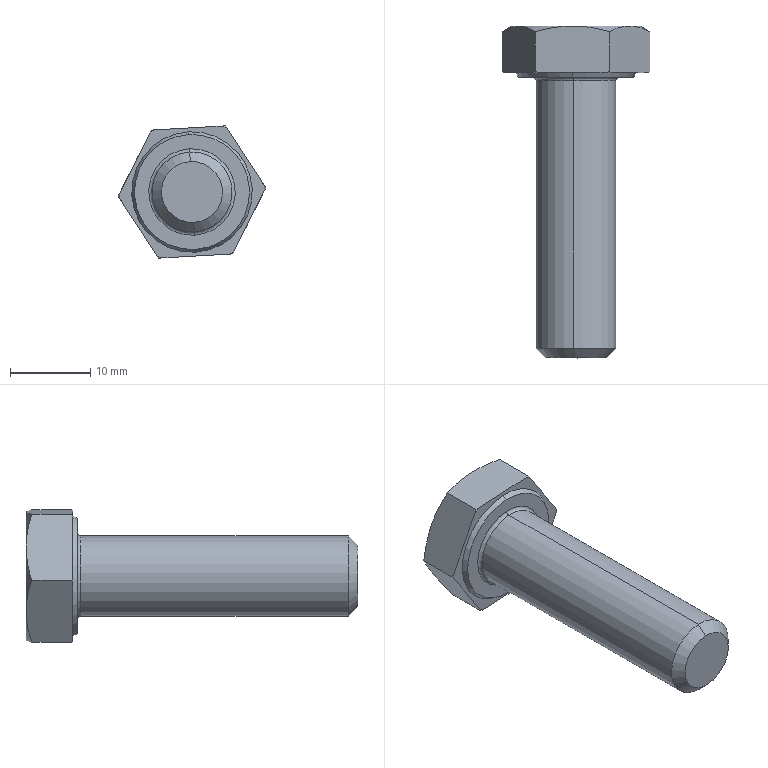Part | STEP file | BFACE2-39 | 1 solid | 30 faces | box 18.445 x 41.4 x 16.5 mm | volume 4112 mm3 | cone 16 | plane 10 | cylinder 2 | torus 2 | commonest cylinder face diameters 10 x2
STEP:
#1=CARTESIAN_POINT('',(-602.523,-427.673,3364.161));
#2=VERTEX_POINT('',#1);
#3=CARTESIAN_POINT('',(-601.954,-427.673,3354.177));
#4=VERTEX_POINT('',#3);
#5=CARTESIAN_POINT('',(-602.238,-427.673,3359.169));
#6=DIRECTION('',(0.,1.,0.));
#7=DIRECTION('',(-0.05688,0.,0.9984));
#8=AXIS2_PLACEMENT_3D('',#5,#6,#7);
#9=CIRCLE('',#8,5.);
#10=EDGE_CURVE('',#2,#4,#9,.T.);
#11=ORIENTED_EDGE('',*,*,#10,.F.);
#12=CARTESIAN_POINT('',(-602.523,-461.073,3364.161));
#13=VERTEX_POINT('',#12);
#14=CARTESIAN_POINT('',(-602.523,-420.873,3364.161));
#15=DIRECTION('',(0.,1.,0.));
#16=VECTOR('',#15,1000.);
#17=LINE('',#14,#16);
#18=EDGE_CURVE('',#13,#2,#17,.T.);
#19=ORIENTED_EDGE('',*,*,#18,.F.);
#20=CARTESIAN_POINT('',(-601.954,-461.073,3354.177));
#21=VERTEX_POINT('',#20);
#22=CARTESIAN_POINT('',(-602.238,-461.073,3359.169));
#23=DIRECTION('',(0.,1.,0.));
#24=DIRECTION('',(0.05688,0.,-0.9984));
#25=AXIS2_PLACEMENT_3D('',#22,#23,#24);
#26=CIRCLE('',#25,5.);
#27=EDGE_CURVE('',#13,#21,#26,.T.);
#28=ORIENTED_EDGE('',*,*,#27,.T.);
#29=CARTESIAN_POINT('',(-601.954,-420.873,3354.177));
#30=DIRECTION('',(0.,1.,0.));
#31=VECTOR('',#30,1000.);
#32=LINE('',#29,#31);
#33=EDGE_CURVE('',#21,#4,#32,.T.);
#34=ORIENTED_EDGE('',*,*,#33,.T.);
#35=EDGE_LOOP('',(#11,#19,#28,#34));
#36=FACE_OUTER_BOUND('',#35,.T.);
#37=CARTESIAN_POINT('',(-602.238,-420.873,3359.169));
#38=DIRECTION('',(0.,-1.,0.));
#39=DIRECTION('',(-0.05688,0.,0.9984));
#40=AXIS2_PLACEMENT_3D('',#37,#38,#39);
#41=CYLINDRICAL_SURFACE('',#40,5.);
#42=ADVANCED_FACE('',(#36),#41,.T.);
#43=CARTESIAN_POINT('',(-602.022,-462.273,3355.375));
#44=VERTEX_POINT('',#43);
#45=CARTESIAN_POINT('',(-602.454,-462.273,3362.963));
#46=VERTEX_POINT('',#45);
#47=CARTESIAN_POINT('',(-602.238,-462.273,3359.169));
#48=DIRECTION('',(0.,-1.,0.));
#49=DIRECTION('',(0.05688,0.,-0.9984));
#50=AXIS2_PLACEMENT_3D('',#47,#48,#49);
#51=CIRCLE('',#50,3.8);
#52=EDGE_CURVE('',#44,#46,#51,.T.);
#53=ORIENTED_EDGE('',*,*,#52,.F.);
#54=CARTESIAN_POINT('',(-602.022,-462.273,3355.375));
#55=DIRECTION('',(0.04022,0.7071,-0.706));
#56=VECTOR('',#55,1000.);
#57=LINE('',#54,#56);
#58=EDGE_CURVE('',#44,#21,#57,.T.);
#59=ORIENTED_EDGE('',*,*,#58,.T.);
#60=ORIENTED_EDGE('',*,*,#27,.F.);
#61=CARTESIAN_POINT('',(-602.454,-462.273,3362.963));
#62=DIRECTION('',(-0.04022,0.7071,0.706));
#63=VECTOR('',#62,1000.);
#64=LINE('',#61,#63);
#65=EDGE_CURVE('',#46,#13,#64,.T.);
#66=ORIENTED_EDGE('',*,*,#65,.F.);
#67=EDGE_LOOP('',(#53,#59,#60,#66));
#68=FACE_OUTER_BOUND('',#67,.T.);
#69=CARTESIAN_POINT('',(-602.238,-462.273,3359.169));
#70=DIRECTION('',(0.,1.,0.));
#71=DIRECTION('',(0.05688,0.,-0.9984));
#72=AXIS2_PLACEMENT_3D('',#69,#70,#71);
#73=CONICAL_SURFACE('',#72,3.8,0.7854);
#74=ADVANCED_FACE('',(#68),#73,.T.);
#75=CARTESIAN_POINT('',(-601.931,-427.273,3353.778));
#76=VERTEX_POINT('',#75);
#77=CARTESIAN_POINT('',(-602.545,-427.273,3364.56));
#78=VERTEX_POINT('',#77);
#79=CARTESIAN_POINT('',(-602.238,-427.273,3359.169));
#80=DIRECTION('',(0.,1.,0.));
#81=DIRECTION('',(-0.05688,0.,0.9984));
#82=AXIS2_PLACEMENT_3D('',#79,#80,#81);
#83=CIRCLE('',#82,5.4);
#84=EDGE_CURVE('',#76,#78,#83,.T.);
#85=ORIENTED_EDGE('',*,*,#84,.F.);
#86=CARTESIAN_POINT('',(-601.931,-427.673,3353.778));
#87=DIRECTION('',(0.9984,0.,0.05688));
#88=DIRECTION('',(-0.05688,0.,0.9984));
#89=AXIS2_PLACEMENT_3D('',#86,#87,#88);
#90=CIRCLE('',#89,0.4);
#91=EDGE_CURVE('',#76,#4,#90,.T.);
#92=ORIENTED_EDGE('',*,*,#91,.T.);
#93=CARTESIAN_POINT('',(-602.238,-427.673,3359.169));
#94=DIRECTION('',(0.,1.,0.));
#95=DIRECTION('',(-0.05688,0.,0.9984));
#96=AXIS2_PLACEMENT_3D('',#93,#94,#95);
#97=CIRCLE('',#96,5.);
#98=EDGE_CURVE('',#4,#2,#97,.T.);
#99=ORIENTED_EDGE('',*,*,#98,.T.);
#100=CARTESIAN_POINT('',(-602.545,-427.673,3364.56));
#101=DIRECTION('',(-0.9984,0.,-0.05688));
#102=DIRECTION('',(0.05688,0.,-0.9984));
#103=AXIS2_PLACEMENT_3D('',#100,#101,#102);
#104=CIRCLE('',#103,0.4);
#105=EDGE_CURVE('',#78,#2,#104,.T.);
#106=ORIENTED_EDGE('',*,*,#105,.F.);
#107=EDGE_LOOP('',(#85,#92,#99,#106));
#108=FACE_OUTER_BOUND('',#107,.T.);
#109=CARTESIAN_POINT('',(-602.238,-427.673,3359.169));
#110=DIRECTION('',(0.,1.,0.));
#111=DIRECTION('',(0.05688,0.,-0.9984));
#112=AXIS2_PLACEMENT_3D('',#109,#110,#111);
#113=TOROIDAL_SURFACE('',#112,5.4,0.4);
#114=ADVANCED_FACE('',(#108),#113,.F.);
#115=CARTESIAN_POINT('',(-602.647,-427.273,3366.335));
#116=VERTEX_POINT('',#115);
#117=CARTESIAN_POINT('',(-601.83,-427.273,3352.003));
#118=VERTEX_POINT('',#117);
#119=CARTESIAN_POINT('',(-602.238,-427.273,3359.169));
#120=DIRECTION('',(0.,1.,0.));
#121=DIRECTION('',(-0.05688,0.,0.9984));
#122=AXIS2_PLACEMENT_3D('',#119,#120,#121);
#123=CIRCLE('',#122,7.177);
#124=EDGE_CURVE('',#116,#118,#123,.T.);
#125=ORIENTED_EDGE('',*,*,#124,.T.);
#126=CARTESIAN_POINT('',(-601.81,-426.673,3351.658));
#127=VERTEX_POINT('',#126);
#128=CARTESIAN_POINT('',(-601.81,-426.673,3351.658));
#129=DIRECTION('',(0.02844,0.866,-0.4992));
#130=VECTOR('',#129,1000.);
#131=LINE('',#128,#130);
#132=EDGE_CURVE('',#118,#127,#131,.T.);
#133=ORIENTED_EDGE('',*,*,#132,.T.);
#134=CARTESIAN_POINT('',(-602.666,-426.673,3366.681));
#135=VERTEX_POINT('',#134);
#136=CARTESIAN_POINT('',(-602.238,-426.673,3359.169));
#137=DIRECTION('',(0.,1.,0.));
#138=DIRECTION('',(-0.05688,0.,0.9984));
#139=AXIS2_PLACEMENT_3D('',#136,#137,#138);
#140=CIRCLE('',#139,7.524);
#141=EDGE_CURVE('',#135,#127,#140,.T.);
#142=ORIENTED_EDGE('',*,*,#141,.F.);
#143=CARTESIAN_POINT('',(-602.666,-426.673,3366.681));
#144=DIRECTION('',(-0.02844,0.866,0.4992));
#145=VECTOR('',#144,1000.);
#146=LINE('',#143,#145);
#147=EDGE_CURVE('',#116,#135,#146,.T.);
#148=ORIENTED_EDGE('',*,*,#147,.F.);
#149=EDGE_LOOP('',(#125,#133,#142,#148));
#150=FACE_OUTER_BOUND('',#149,.T.);
#151=CARTESIAN_POINT('',(-602.238,-426.673,3359.169));
#152=DIRECTION('',(0.,1.,0.));
#153=DIRECTION('',(0.05688,0.,-0.9984));
#154=AXIS2_PLACEMENT_3D('',#151,#152,#153);
#155=CONICAL_SURFACE('',#154,7.524,0.5236);
#156=ADVANCED_FACE('',(#150),#155,.T.);
#157=ORIENTED_EDGE('',*,*,#124,.F.);
#158=CARTESIAN_POINT('',(-602.238,-427.273,3359.169));
#159=DIRECTION('',(0.,1.,0.));
#160=DIRECTION('',(-0.05688,0.,0.9984));
#161=AXIS2_PLACEMENT_3D('',#158,#159,#160);
#162=CIRCLE('',#161,7.177);
#163=EDGE_CURVE('',#118,#116,#162,.T.);
#164=ORIENTED_EDGE('',*,*,#163,.F.);
#165=EDGE_LOOP('',(#157,#164));
#166=FACE_OUTER_BOUND('',#165,.T.);
#167=CARTESIAN_POINT('',(-602.238,-427.273,3359.169));
#168=DIRECTION('',(0.,1.,0.));
#169=DIRECTION('',(-0.05688,0.,0.9984));
#170=AXIS2_PLACEMENT_3D('',#167,#168,#169);
#171=CIRCLE('',#170,5.4);
#172=EDGE_CURVE('',#78,#76,#171,.T.);
#173=ORIENTED_EDGE('',*,*,#172,.T.);
#174=ORIENTED_EDGE('',*,*,#84,.T.);
#175=EDGE_LOOP('',(#173,#174));
#176=FACE_BOUND('',#175,.T.);
#177=CARTESIAN_POINT('',(-593.016,-427.273,3359.695));
#178=DIRECTION('',(0.,-1.,0.));
#179=DIRECTION('',(-0.05688,0.,0.9984));
#180=AXIS2_PLACEMENT_3D('',#177,#178,#179);
#181=PLANE('',#180);
#182=ADVANCED_FACE('',(#166,#176),#181,.T.);
#183=CARTESIAN_POINT('',(-596.987,-426.673,3351.812));
#184=VERTEX_POINT('',#183);
#185=CARTESIAN_POINT('',(-593.2,-426.673,3359.328));
#186=VERTEX_POINT('',#185);
#187=CARTESIAN_POINT('',(-597.172,-426.673,3351.445));
#188=DIRECTION('',(0.4499,0.,0.8931));
#189=VECTOR('',#188,1000.);
#190=LINE('',#187,#189);
#191=EDGE_CURVE('',#184,#186,#190,.T.);
#192=ORIENTED_EDGE('',*,*,#191,.F.);
#193=CARTESIAN_POINT('',(-597.172,-426.559,3351.445));
#194=VERTEX_POINT('',#193);
#195=CARTESIAN_POINT('',(-597.172,-426.559,3351.445));
#196=CARTESIAN_POINT('',(-597.11,-426.598,3351.567));
#197=CARTESIAN_POINT('',(-597.049,-426.636,3351.689));
#198=CARTESIAN_POINT('',(-596.987,-426.673,3351.812));
#199=B_SPLINE_CURVE_WITH_KNOTS('',3,(#195,#196,#197,#198),.UNSPECIFIED.,.F.,.F.,(4,4),(0.,1.),.UNSPECIFIED.);
#200=EDGE_CURVE('',#194,#184,#199,.T.);
#201=ORIENTED_EDGE('',*,*,#200,.F.);
#202=CARTESIAN_POINT('',(-597.172,-421.588,3351.445));
#203=VERTEX_POINT('',#202);
#204=CARTESIAN_POINT('',(-597.172,-427.273,3351.445));
#205=DIRECTION('',(0.,1.,0.));
#206=VECTOR('',#205,1000.);
#207=LINE('',#204,#206);
#208=EDGE_CURVE('',#194,#203,#207,.T.);
#209=ORIENTED_EDGE('',*,*,#208,.T.);
#210=CARTESIAN_POINT('',(-595.094,-420.873,3355.57));
#211=VERTEX_POINT('',#210);
#212=CARTESIAN_POINT('',(-595.094,-420.873,3355.57));
#213=CARTESIAN_POINT('',(-595.448,-420.873,3354.866));
#214=CARTESIAN_POINT('',(-595.798,-420.941,3354.171));
#215=CARTESIAN_POINT('',(-596.49,-421.19,3352.798));
#216=CARTESIAN_POINT('',(-596.832,-421.37,3352.119));
#217=CARTESIAN_POINT('',(-597.172,-421.588,3351.445));
#218=B_SPLINE_CURVE_WITH_KNOTS('',3,(#212,#213,#214,#215,#216,#217),.UNSPECIFIED.,.F.,.F.,(4,2,4),(0.,0.002337,0.004674),.UNSPECIFIED.);
#219=EDGE_CURVE('',#211,#203,#218,.T.);
#220=ORIENTED_EDGE('',*,*,#219,.F.);
#221=CARTESIAN_POINT('',(-593.016,-421.588,3359.695));
#222=VERTEX_POINT('',#221);
#223=CARTESIAN_POINT('',(-593.016,-421.588,3359.695));
#224=CARTESIAN_POINT('',(-593.355,-421.37,3359.021));
#225=CARTESIAN_POINT('',(-593.697,-421.19,3358.342));
#226=CARTESIAN_POINT('',(-594.389,-420.941,3356.968));
#227=CARTESIAN_POINT('',(-594.739,-420.873,3356.274));
#228=CARTESIAN_POINT('',(-595.094,-420.873,3355.57));
#229=B_SPLINE_CURVE_WITH_KNOTS('',3,(#223,#224,#225,#226,#227,#228),.UNSPECIFIED.,.F.,.F.,(4,2,4),(0.,0.002337,0.004674),.UNSPECIFIED.);
#230=EDGE_CURVE('',#222,#211,#229,.T.);
#231=ORIENTED_EDGE('',*,*,#230,.F.);
#232=CARTESIAN_POINT('',(-593.016,-426.559,3359.695));
#233=VERTEX_POINT('',#232);
#234=CARTESIAN_POINT('',(-593.016,-427.273,3359.695));
#235=DIRECTION('',(0.,1.,0.));
#236=VECTOR('',#235,1000.);
#237=LINE('',#234,#236);
#238=EDGE_CURVE('',#233,#222,#237,.T.);
#239=ORIENTED_EDGE('',*,*,#238,.F.);
#240=CARTESIAN_POINT('',(-593.2,-426.673,3359.328));
#241=CARTESIAN_POINT('',(-593.139,-426.636,3359.45));
#242=CARTESIAN_POINT('',(-593.077,-426.598,3359.572));
#243=CARTESIAN_POINT('',(-593.016,-426.559,3359.695));
#244=B_SPLINE_CURVE_WITH_KNOTS('',3,(#240,#241,#242,#243),.UNSPECIFIED.,.F.,.F.,(4,4),(0.,1.),.UNSPECIFIED.);
#245=EDGE_CURVE('',#186,#233,#244,.T.);
#246=ORIENTED_EDGE('',*,*,#245,.F.);
#247=EDGE_LOOP('',(#192,#201,#209,#220,#231,#239,#246));
#248=FACE_OUTER_BOUND('',#247,.T.);
#249=CARTESIAN_POINT('',(-597.172,-427.273,3351.445));
#250=DIRECTION('',(-0.8931,0.,0.4499));
#251=DIRECTION('',(0.4499,0.,0.8931));
#252=AXIS2_PLACEMENT_3D('',#249,#250,#251);
#253=PLANE('',#252);
#254=ADVANCED_FACE('',(#248),#253,.F.);
#255=CARTESIAN_POINT('',(-593.241,-426.673,3360.038));
#256=VERTEX_POINT('',#255);
#257=CARTESIAN_POINT('',(-597.857,-426.673,3367.075));
#258=VERTEX_POINT('',#257);
#259=CARTESIAN_POINT('',(-593.016,-426.673,3359.695));
#260=DIRECTION('',(-0.5485,0.,0.8362));
#261=VECTOR('',#260,1000.);
#262=LINE('',#259,#261);
#263=EDGE_CURVE('',#256,#258,#262,.T.);
#264=ORIENTED_EDGE('',*,*,#263,.F.);
#265=CARTESIAN_POINT('',(-593.016,-426.559,3359.695));
#266=CARTESIAN_POINT('',(-593.091,-426.598,3359.809));
#267=CARTESIAN_POINT('',(-593.166,-426.636,3359.923));
#268=CARTESIAN_POINT('',(-593.241,-426.673,3360.038));
#269=B_SPLINE_CURVE_WITH_KNOTS('',3,(#265,#266,#267,#268),.UNSPECIFIED.,.F.,.F.,(4,4),(0.,1.),.UNSPECIFIED.);
#270=EDGE_CURVE('',#233,#256,#269,.T.);
#271=ORIENTED_EDGE('',*,*,#270,.F.);
#272=ORIENTED_EDGE('',*,*,#238,.T.);
#273=CARTESIAN_POINT('',(-595.549,-420.873,3363.557));
#274=VERTEX_POINT('',#273);
#275=CARTESIAN_POINT('',(-595.549,-420.873,3363.557));
#276=CARTESIAN_POINT('',(-595.117,-420.873,3362.898));
#277=CARTESIAN_POINT('',(-594.69,-420.941,3362.247));
#278=CARTESIAN_POINT('',(-593.847,-421.19,3360.961));
#279=CARTESIAN_POINT('',(-593.429,-421.37,3360.325));
#280=CARTESIAN_POINT('',(-593.016,-421.588,3359.695));
#281=B_SPLINE_CURVE_WITH_KNOTS('',3,(#275,#276,#277,#278,#279,#280),.UNSPECIFIED.,.F.,.F.,(4,2,4),(0.,0.002337,0.004674),.UNSPECIFIED.);
#282=EDGE_CURVE('',#274,#222,#281,.T.);
#283=ORIENTED_EDGE('',*,*,#282,.F.);
#284=CARTESIAN_POINT('',(-598.082,-421.588,3367.419));
#285=VERTEX_POINT('',#284);
#286=CARTESIAN_POINT('',(-598.082,-421.588,3367.419));
#287=CARTESIAN_POINT('',(-597.668,-421.37,3366.788));
#288=CARTESIAN_POINT('',(-597.251,-421.19,3366.152));
#289=CARTESIAN_POINT('',(-596.408,-420.941,3364.866));
#290=CARTESIAN_POINT('',(-595.981,-420.873,3364.216));
#291=CARTESIAN_POINT('',(-595.549,-420.873,3363.557));
#292=B_SPLINE_CURVE_WITH_KNOTS('',3,(#286,#287,#288,#289,#290,#291),.UNSPECIFIED.,.F.,.F.,(4,2,4),(0.,0.002337,0.004674),.UNSPECIFIED.);
#293=EDGE_CURVE('',#285,#274,#292,.T.);
#294=ORIENTED_EDGE('',*,*,#293,.F.);
#295=CARTESIAN_POINT('',(-598.082,-426.559,3367.419));
#296=VERTEX_POINT('',#295);
#297=CARTESIAN_POINT('',(-598.082,-427.273,3367.419));
#298=DIRECTION('',(0.,1.,0.));
#299=VECTOR('',#298,1000.);
#300=LINE('',#297,#299);
#301=EDGE_CURVE('',#296,#285,#300,.T.);
#302=ORIENTED_EDGE('',*,*,#301,.F.);
#303=CARTESIAN_POINT('',(-597.857,-426.673,3367.075));
#304=CARTESIAN_POINT('',(-597.932,-426.636,3367.19));
#305=CARTESIAN_POINT('',(-598.007,-426.598,3367.305));
#306=CARTESIAN_POINT('',(-598.082,-426.559,3367.419));
#307=B_SPLINE_CURVE_WITH_KNOTS('',3,(#303,#304,#305,#306),.UNSPECIFIED.,.F.,.F.,(4,4),(0.,1.),.UNSPECIFIED.);
#308=EDGE_CURVE('',#258,#296,#307,.T.);
#309=ORIENTED_EDGE('',*,*,#308,.F.);
#310=EDGE_LOOP('',(#264,#271,#272,#283,#294,#302,#309));
#311=FACE_OUTER_BOUND('',#310,.T.);
#312=CARTESIAN_POINT('',(-593.016,-427.273,3359.695));
#313=DIRECTION('',(-0.8362,0.,-0.5485));
#314=DIRECTION('',(-0.5485,0.,0.8362));
#315=AXIS2_PLACEMENT_3D('',#312,#313,#314);
#316=PLANE('',#315);
#317=ADVANCED_FACE('',(#311),#316,.F.);
#318=CARTESIAN_POINT('',(-598.492,-426.673,3367.395));
#319=VERTEX_POINT('',#318);
#320=CARTESIAN_POINT('',(-606.895,-426.673,3366.917));
#321=VERTEX_POINT('',#320);
#322=CARTESIAN_POINT('',(-598.082,-426.673,3367.419));
#323=DIRECTION('',(-0.9984,0.,-0.05688));
#324=VECTOR('',#323,1000.);
#325=LINE('',#322,#324);
#326=EDGE_CURVE('',#319,#321,#325,.T.);
#327=ORIENTED_EDGE('',*,*,#326,.F.);
#328=CARTESIAN_POINT('',(-598.082,-426.559,3367.419));
#329=CARTESIAN_POINT('',(-598.218,-426.598,3367.411));
#330=CARTESIAN_POINT('',(-598.355,-426.636,3367.403));
#331=CARTESIAN_POINT('',(-598.492,-426.673,3367.395));
#332=B_SPLINE_CURVE_WITH_KNOTS('',3,(#328,#329,#330,#331),.UNSPECIFIED.,.F.,.F.,(4,4),(0.,1.),.UNSPECIFIED.);
#333=EDGE_CURVE('',#296,#319,#332,.T.);
#334=ORIENTED_EDGE('',*,*,#333,.F.);
#335=ORIENTED_EDGE('',*,*,#301,.T.);
#336=CARTESIAN_POINT('',(-602.693,-420.873,3367.156));
#337=VERTEX_POINT('',#336);
#338=CARTESIAN_POINT('',(-602.693,-420.873,3367.156));
#339=CARTESIAN_POINT('',(-601.906,-420.873,3367.201));
#340=CARTESIAN_POINT('',(-601.13,-420.941,3367.245));
#341=CARTESIAN_POINT('',(-599.595,-421.19,3367.333));
#342=CARTESIAN_POINT('',(-598.835,-421.37,3367.376));
#343=CARTESIAN_POINT('',(-598.082,-421.588,3367.419));
#344=B_SPLINE_CURVE_WITH_KNOTS('',3,(#338,#339,#340,#341,#342,#343),.UNSPECIFIED.,.F.,.F.,(4,2,4),(0.,0.002337,0.004674),.UNSPECIFIED.);
#345=EDGE_CURVE('',#337,#285,#344,.T.);
#346=ORIENTED_EDGE('',*,*,#345,.F.);
#347=CARTESIAN_POINT('',(-607.305,-421.588,3366.893));
#348=VERTEX_POINT('',#347);
#349=CARTESIAN_POINT('',(-607.305,-421.588,3366.893));
#350=CARTESIAN_POINT('',(-606.551,-421.37,3366.936));
#351=CARTESIAN_POINT('',(-605.792,-421.19,3366.98));
#352=CARTESIAN_POINT('',(-604.257,-420.941,3367.067));
#353=CARTESIAN_POINT('',(-603.48,-420.873,3367.111));
#354=CARTESIAN_POINT('',(-602.693,-420.873,3367.156));
#355=B_SPLINE_CURVE_WITH_KNOTS('',3,(#349,#350,#351,#352,#353,#354),.UNSPECIFIED.,.F.,.F.,(4,2,4),(0.,0.002337,0.004674),.UNSPECIFIED.);
#356=EDGE_CURVE('',#348,#337,#355,.T.);
#357=ORIENTED_EDGE('',*,*,#356,.F.);
#358=CARTESIAN_POINT('',(-607.305,-426.559,3366.893));
#359=VERTEX_POINT('',#358);
#360=CARTESIAN_POINT('',(-607.305,-427.273,3366.893));
#361=DIRECTION('',(0.,1.,0.));
#362=VECTOR('',#361,1000.);
#363=LINE('',#360,#362);
#364=EDGE_CURVE('',#359,#348,#363,.T.);
#365=ORIENTED_EDGE('',*,*,#364,.F.);
#366=CARTESIAN_POINT('',(-606.895,-426.673,3366.917));
#367=CARTESIAN_POINT('',(-607.032,-426.636,3366.909));
#368=CARTESIAN_POINT('',(-607.168,-426.598,3366.901));
#369=CARTESIAN_POINT('',(-607.305,-426.559,3366.893));
#370=B_SPLINE_CURVE_WITH_KNOTS('',3,(#366,#367,#368,#369),.UNSPECIFIED.,.F.,.F.,(4,4),(0.,1.),.UNSPECIFIED.);
#371=EDGE_CURVE('',#321,#359,#370,.T.);
#372=ORIENTED_EDGE('',*,*,#371,.F.);
#373=EDGE_LOOP('',(#327,#334,#335,#346,#357,#365,#372));
#374=FACE_OUTER_BOUND('',#373,.T.);
#375=CARTESIAN_POINT('',(-598.082,-427.273,3367.419));
#376=DIRECTION('',(0.05688,0.,-0.9984));
#377=DIRECTION('',(0.,-1.,0.));
#378=AXIS2_PLACEMENT_3D('',#375,#376,#377);
#379=PLANE('',#378);
#380=ADVANCED_FACE('',(#374),#379,.F.);
#381=CARTESIAN_POINT('',(-607.489,-426.673,3366.527));
#382=VERTEX_POINT('',#381);
#383=CARTESIAN_POINT('',(-611.276,-426.673,3359.01));
#384=VERTEX_POINT('',#383);
#385=CARTESIAN_POINT('',(-611.461,-426.673,3358.644));
#386=DIRECTION('',(-0.4499,0.,-0.8931));
#387=VECTOR('',#386,1000.);
#388=LINE('',#385,#387);
#389=EDGE_CURVE('',#382,#384,#388,.T.);
#390=ORIENTED_EDGE('',*,*,#389,.F.);
#391=CARTESIAN_POINT('',(-607.305,-426.559,3366.893));
#392=CARTESIAN_POINT('',(-607.366,-426.598,3366.771));
#393=CARTESIAN_POINT('',(-607.428,-426.636,3366.649));
#394=CARTESIAN_POINT('',(-607.489,-426.673,3366.527));
#395=B_SPLINE_CURVE_WITH_KNOTS('',3,(#391,#392,#393,#394),.UNSPECIFIED.,.F.,.F.,(4,4),(0.,1.),.UNSPECIFIED.);
#396=EDGE_CURVE('',#359,#382,#395,.T.);
#397=ORIENTED_EDGE('',*,*,#396,.F.);
#398=ORIENTED_EDGE('',*,*,#364,.T.);
#399=CARTESIAN_POINT('',(-609.383,-420.873,3362.768));
#400=VERTEX_POINT('',#399);
#401=CARTESIAN_POINT('',(-609.383,-420.873,3362.768));
#402=CARTESIAN_POINT('',(-609.028,-420.873,3363.472));
#403=CARTESIAN_POINT('',(-608.678,-420.941,3364.167));
#404=CARTESIAN_POINT('',(-607.986,-421.19,3365.54));
#405=CARTESIAN_POINT('',(-607.644,-421.37,3366.22));
#406=CARTESIAN_POINT('',(-607.305,-421.588,3366.893));
#407=B_SPLINE_CURVE_WITH_KNOTS('',3,(#401,#402,#403,#404,#405,#406),.UNSPECIFIED.,.F.,.F.,(4,2,4),(0.,0.002337,0.004674),.UNSPECIFIED.);
#408=EDGE_CURVE('',#400,#348,#407,.T.);
#409=ORIENTED_EDGE('',*,*,#408,.F.);
#410=CARTESIAN_POINT('',(-611.461,-421.588,3358.644));
#411=VERTEX_POINT('',#410);
#412=CARTESIAN_POINT('',(-611.461,-421.588,3358.644));
#413=CARTESIAN_POINT('',(-611.121,-421.37,3359.317));
#414=CARTESIAN_POINT('',(-610.779,-421.19,3359.997));
#415=CARTESIAN_POINT('',(-610.087,-420.941,3361.37));
#416=CARTESIAN_POINT('',(-609.737,-420.873,3362.065));
#417=CARTESIAN_POINT('',(-609.383,-420.873,3362.768));
#418=B_SPLINE_CURVE_WITH_KNOTS('',3,(#412,#413,#414,#415,#416,#417),.UNSPECIFIED.,.F.,.F.,(4,2,4),(0.,0.002337,0.004674),.UNSPECIFIED.);
#419=EDGE_CURVE('',#411,#400,#418,.T.);
#420=ORIENTED_EDGE('',*,*,#419,.F.);
#421=CARTESIAN_POINT('',(-611.461,-426.559,3358.644));
#422=VERTEX_POINT('',#421);
#423=CARTESIAN_POINT('',(-611.461,-427.273,3358.644));
#424=DIRECTION('',(0.,1.,0.));
#425=VECTOR('',#424,1000.);
#426=LINE('',#423,#425);
#427=EDGE_CURVE('',#422,#411,#426,.T.);
#428=ORIENTED_EDGE('',*,*,#427,.F.);
#429=CARTESIAN_POINT('',(-611.276,-426.673,3359.01));
#430=CARTESIAN_POINT('',(-611.338,-426.636,3358.888));
#431=CARTESIAN_POINT('',(-611.399,-426.598,3358.766));
#432=CARTESIAN_POINT('',(-611.461,-426.559,3358.644));
#433=B_SPLINE_CURVE_WITH_KNOTS('',3,(#429,#430,#431,#432),.UNSPECIFIED.,.F.,.F.,(4,4),(0.,1.),.UNSPECIFIED.);
#434=EDGE_CURVE('',#384,#422,#433,.T.);
#435=ORIENTED_EDGE('',*,*,#434,.F.);
#436=EDGE_LOOP('',(#390,#397,#398,#409,#420,#428,#435));
#437=FACE_OUTER_BOUND('',#436,.T.);
#438=CARTESIAN_POINT('',(-611.461,-427.273,3358.644));
#439=DIRECTION('',(0.8931,0.,-0.4499));
#440=DIRECTION('',(-0.4499,0.,-0.8931));
#441=AXIS2_PLACEMENT_3D('',#438,#439,#440);
#442=PLANE('',#441);
#443=ADVANCED_FACE('',(#437),#442,.F.);
#444=CARTESIAN_POINT('',(-611.236,-426.673,3358.3));
#445=VERTEX_POINT('',#444);
#446=CARTESIAN_POINT('',(-606.62,-426.673,3351.263));
#447=VERTEX_POINT('',#446);
#448=CARTESIAN_POINT('',(-606.395,-426.673,3350.919));
#449=DIRECTION('',(0.5485,0.,-0.8362));
#450=VECTOR('',#449,1000.);
#451=LINE('',#448,#450);
#452=EDGE_CURVE('',#445,#447,#451,.T.);
#453=ORIENTED_EDGE('',*,*,#452,.F.);
#454=CARTESIAN_POINT('',(-611.461,-426.559,3358.644));
#455=CARTESIAN_POINT('',(-611.386,-426.598,3358.529));
#456=CARTESIAN_POINT('',(-611.311,-426.636,3358.415));
#457=CARTESIAN_POINT('',(-611.236,-426.673,3358.3));
#458=B_SPLINE_CURVE_WITH_KNOTS('',3,(#454,#455,#456,#457),.UNSPECIFIED.,.F.,.F.,(4,4),(0.,1.),.UNSPECIFIED.);
#459=EDGE_CURVE('',#422,#445,#458,.T.);
#460=ORIENTED_EDGE('',*,*,#459,.F.);
#461=ORIENTED_EDGE('',*,*,#427,.T.);
#462=CARTESIAN_POINT('',(-608.928,-420.873,3354.781));
#463=VERTEX_POINT('',#462);
#464=CARTESIAN_POINT('',(-608.928,-420.873,3354.781));
#465=CARTESIAN_POINT('',(-609.36,-420.873,3355.441));
#466=CARTESIAN_POINT('',(-609.787,-420.941,3356.091));
#467=CARTESIAN_POINT('',(-610.63,-421.19,3357.377));
#468=CARTESIAN_POINT('',(-611.047,-421.37,3358.013));
#469=CARTESIAN_POINT('',(-611.461,-421.588,3358.644));
#470=B_SPLINE_CURVE_WITH_KNOTS('',3,(#464,#465,#466,#467,#468,#469),.UNSPECIFIED.,.F.,.F.,(4,2,4),(0.,0.002337,0.004674),.UNSPECIFIED.);
#471=EDGE_CURVE('',#463,#411,#470,.T.);
#472=ORIENTED_EDGE('',*,*,#471,.F.);
#473=CARTESIAN_POINT('',(-606.395,-421.588,3350.919));
#474=VERTEX_POINT('',#473);
#475=CARTESIAN_POINT('',(-606.395,-421.588,3350.919));
#476=CARTESIAN_POINT('',(-606.808,-421.37,3351.55));
#477=CARTESIAN_POINT('',(-607.225,-421.19,3352.186));
#478=CARTESIAN_POINT('',(-608.069,-420.941,3353.472));
#479=CARTESIAN_POINT('',(-608.495,-420.873,3354.122));
#480=CARTESIAN_POINT('',(-608.928,-420.873,3354.781));
#481=B_SPLINE_CURVE_WITH_KNOTS('',3,(#475,#476,#477,#478,#479,#480),.UNSPECIFIED.,.F.,.F.,(4,2,4),(0.,0.002337,0.004674),.UNSPECIFIED.);
#482=EDGE_CURVE('',#474,#463,#481,.T.);
#483=ORIENTED_EDGE('',*,*,#482,.F.);
#484=CARTESIAN_POINT('',(-606.395,-426.559,3350.919));
#485=VERTEX_POINT('',#484);
#486=CARTESIAN_POINT('',(-606.395,-427.273,3350.919));
#487=DIRECTION('',(0.,1.,0.));
#488=VECTOR('',#487,1000.);
#489=LINE('',#486,#488);
#490=EDGE_CURVE('',#485,#474,#489,.T.);
#491=ORIENTED_EDGE('',*,*,#490,.F.);
#492=CARTESIAN_POINT('',(-606.62,-426.673,3351.263));
#493=CARTESIAN_POINT('',(-606.545,-426.636,3351.148));
#494=CARTESIAN_POINT('',(-606.469,-426.598,3351.034));
#495=CARTESIAN_POINT('',(-606.395,-426.559,3350.919));
#496=B_SPLINE_CURVE_WITH_KNOTS('',3,(#492,#493,#494,#495),.UNSPECIFIED.,.F.,.F.,(4,4),(0.,1.),.UNSPECIFIED.);
#497=EDGE_CURVE('',#447,#485,#496,.T.);
#498=ORIENTED_EDGE('',*,*,#497,.F.);
#499=EDGE_LOOP('',(#453,#460,#461,#472,#483,#491,#498));
#500=FACE_OUTER_BOUND('',#499,.T.);
#501=CARTESIAN_POINT('',(-606.395,-427.273,3350.919));
#502=DIRECTION('',(0.8362,0.,0.5485));
#503=DIRECTION('',(0.5485,0.,-0.8362));
#504=AXIS2_PLACEMENT_3D('',#501,#502,#503);
#505=PLANE('',#504);
#506=ADVANCED_FACE('',(#500),#505,.F.);
#507=CARTESIAN_POINT('',(-605.984,-426.673,3350.943));
#508=VERTEX_POINT('',#507);
#509=CARTESIAN_POINT('',(-597.582,-426.673,3351.421));
#510=VERTEX_POINT('',#509);
#511=CARTESIAN_POINT('',(-597.172,-426.673,3351.445));
#512=DIRECTION('',(0.9984,0.,0.05688));
#513=VECTOR('',#512,1000.);
#514=LINE('',#511,#513);
#515=EDGE_CURVE('',#508,#510,#514,.T.);
#516=ORIENTED_EDGE('',*,*,#515,.F.);
#517=CARTESIAN_POINT('',(-606.395,-426.559,3350.919));
#518=CARTESIAN_POINT('',(-606.258,-426.598,3350.927));
#519=CARTESIAN_POINT('',(-606.122,-426.636,3350.935));
#520=CARTESIAN_POINT('',(-605.984,-426.673,3350.943));
#521=B_SPLINE_CURVE_WITH_KNOTS('',3,(#517,#518,#519,#520),.UNSPECIFIED.,.F.,.F.,(4,4),(0.,1.),.UNSPECIFIED.);
#522=EDGE_CURVE('',#485,#508,#521,.T.);
#523=ORIENTED_EDGE('',*,*,#522,.F.);
#524=ORIENTED_EDGE('',*,*,#490,.T.);
#525=CARTESIAN_POINT('',(-601.783,-420.873,3351.182));
#526=VERTEX_POINT('',#525);
#527=CARTESIAN_POINT('',(-601.783,-420.873,3351.182));
#528=CARTESIAN_POINT('',(-602.57,-420.873,3351.137));
#529=CARTESIAN_POINT('',(-603.347,-420.941,3351.093));
#530=CARTESIAN_POINT('',(-604.882,-421.19,3351.005));
#531=CARTESIAN_POINT('',(-605.641,-421.37,3350.962));
#532=CARTESIAN_POINT('',(-606.395,-421.588,3350.919));
#533=B_SPLINE_CURVE_WITH_KNOTS('',3,(#527,#528,#529,#530,#531,#532),.UNSPECIFIED.,.F.,.F.,(4,2,4),(0.,0.002337,0.004674),.UNSPECIFIED.);
#534=EDGE_CURVE('',#526,#474,#533,.T.);
#535=ORIENTED_EDGE('',*,*,#534,.F.);
#536=CARTESIAN_POINT('',(-597.172,-421.588,3351.445));
#537=CARTESIAN_POINT('',(-597.925,-421.37,3351.402));
#538=CARTESIAN_POINT('',(-598.684,-421.19,3351.359));
#539=CARTESIAN_POINT('',(-600.22,-420.941,3351.271));
#540=CARTESIAN_POINT('',(-600.996,-420.873,3351.227));
#541=CARTESIAN_POINT('',(-601.783,-420.873,3351.182));
#542=B_SPLINE_CURVE_WITH_KNOTS('',3,(#536,#537,#538,#539,#540,#541),.UNSPECIFIED.,.F.,.F.,(4,2,4),(0.,0.002337,0.004674),.UNSPECIFIED.);
#543=EDGE_CURVE('',#203,#526,#542,.T.);
#544=ORIENTED_EDGE('',*,*,#543,.F.);
#545=ORIENTED_EDGE('',*,*,#208,.F.);
#546=CARTESIAN_POINT('',(-597.582,-426.673,3351.421));
#547=CARTESIAN_POINT('',(-597.445,-426.636,3351.429));
#548=CARTESIAN_POINT('',(-597.308,-426.598,3351.437));
#549=CARTESIAN_POINT('',(-597.172,-426.559,3351.445));
#550=B_SPLINE_CURVE_WITH_KNOTS('',3,(#546,#547,#548,#549),.UNSPECIFIED.,.F.,.F.,(4,4),(0.,1.),.UNSPECIFIED.);
#551=EDGE_CURVE('',#510,#194,#550,.T.);
#552=ORIENTED_EDGE('',*,*,#551,.F.);
#553=EDGE_LOOP('',(#516,#523,#524,#535,#544,#545,#552));
#554=FACE_OUTER_BOUND('',#553,.T.);
#555=CARTESIAN_POINT('',(-597.172,-427.273,3351.445));
#556=DIRECTION('',(-0.05688,0.,0.9984));
#557=DIRECTION('',(0.,1.,0.));
#558=AXIS2_PLACEMENT_3D('',#555,#556,#557);
#559=PLANE('',#558);
#560=ADVANCED_FACE('',(#554),#559,.F.);
#561=ORIENTED_EDGE('',*,*,#522,.T.);
#562=CARTESIAN_POINT('',(-602.238,-426.673,3359.169));
#563=DIRECTION('',(0.,1.,0.));
#564=DIRECTION('',(0.05688,0.,-0.9984));
#565=AXIS2_PLACEMENT_3D('',#562,#563,#564);
#566=CIRCLE('',#565,9.039);
#567=EDGE_CURVE('',#508,#447,#566,.T.);
#568=ORIENTED_EDGE('',*,*,#567,.T.);
#569=ORIENTED_EDGE('',*,*,#497,.T.);
#570=EDGE_LOOP('',(#561,#568,#569));
#571=FACE_OUTER_BOUND('',#570,.T.);
#572=CARTESIAN_POINT('',(-602.238,-423.672,3359.169));
#573=DIRECTION('',(0.,1.,0.));
#574=DIRECTION('',(0.05688,0.,-0.9984));
#575=AXIS2_PLACEMENT_3D('',#572,#573,#574);
#576=CONICAL_SURFACE('',#575,14.238,1.047);
#577=ADVANCED_FACE('',(#571),#576,.T.);
#578=ORIENTED_EDGE('',*,*,#459,.T.);
#579=CARTESIAN_POINT('',(-602.238,-426.673,3359.169));
#580=DIRECTION('',(0.,1.,0.));
#581=DIRECTION('',(0.05688,0.,-0.9984));
#582=AXIS2_PLACEMENT_3D('',#579,#580,#581);
#583=CIRCLE('',#582,9.039);
#584=EDGE_CURVE('',#445,#384,#583,.T.);
#585=ORIENTED_EDGE('',*,*,#584,.T.);
#586=ORIENTED_EDGE('',*,*,#434,.T.);
#587=EDGE_LOOP('',(#578,#585,#586));
#588=FACE_OUTER_BOUND('',#587,.T.);
#589=CARTESIAN_POINT('',(-602.238,-423.672,3359.169));
#590=DIRECTION('',(0.,1.,0.));
#591=DIRECTION('',(0.05688,0.,-0.9984));
#592=AXIS2_PLACEMENT_3D('',#589,#590,#591);
#593=CONICAL_SURFACE('',#592,14.238,1.047);
#594=ADVANCED_FACE('',(#588),#593,.T.);
#595=ORIENTED_EDGE('',*,*,#396,.T.);
#596=CARTESIAN_POINT('',(-602.238,-426.673,3359.169));
#597=DIRECTION('',(0.,1.,0.));
#598=DIRECTION('',(0.05688,0.,-0.9984));
#599=AXIS2_PLACEMENT_3D('',#596,#597,#598);
#600=CIRCLE('',#599,9.039);
#601=EDGE_CURVE('',#382,#321,#600,.T.);
#602=ORIENTED_EDGE('',*,*,#601,.T.);
#603=ORIENTED_EDGE('',*,*,#371,.T.);
#604=EDGE_LOOP('',(#595,#602,#603));
#605=FACE_OUTER_BOUND('',#604,.T.);
#606=CARTESIAN_POINT('',(-602.238,-423.672,3359.169));
#607=DIRECTION('',(0.,1.,0.));
#608=DIRECTION('',(0.05688,0.,-0.9984));
#609=AXIS2_PLACEMENT_3D('',#606,#607,#608);
#610=CONICAL_SURFACE('',#609,14.238,1.047);
#611=ADVANCED_FACE('',(#605),#610,.T.);
#612=ORIENTED_EDGE('',*,*,#333,.T.);
#613=CARTESIAN_POINT('',(-602.238,-426.673,3359.169));
#614=DIRECTION('',(0.,1.,0.));
#615=DIRECTION('',(0.05688,0.,-0.9984));
#616=AXIS2_PLACEMENT_3D('',#613,#614,#615);
#617=CIRCLE('',#616,9.039);
#618=EDGE_CURVE('',#319,#258,#617,.T.);
#619=ORIENTED_EDGE('',*,*,#618,.T.);
#620=ORIENTED_EDGE('',*,*,#308,.T.);
#621=EDGE_LOOP('',(#612,#619,#620));
#622=FACE_OUTER_BOUND('',#621,.T.);
#623=CARTESIAN_POINT('',(-602.238,-423.672,3359.169));
#624=DIRECTION('',(0.,1.,0.));
#625=DIRECTION('',(0.05688,0.,-0.9984));
#626=AXIS2_PLACEMENT_3D('',#623,#624,#625);
#627=CONICAL_SURFACE('',#626,14.238,1.047);
#628=ADVANCED_FACE('',(#622),#627,.T.);
#629=ORIENTED_EDGE('',*,*,#270,.T.);
#630=CARTESIAN_POINT('',(-602.238,-426.673,3359.169));
#631=DIRECTION('',(0.,1.,0.));
#632=DIRECTION('',(0.05688,0.,-0.9984));
#633=AXIS2_PLACEMENT_3D('',#630,#631,#632);
#634=CIRCLE('',#633,9.039);
#635=EDGE_CURVE('',#256,#186,#634,.T.);
#636=ORIENTED_EDGE('',*,*,#635,.T.);
#637=ORIENTED_EDGE('',*,*,#245,.T.);
#638=EDGE_LOOP('',(#629,#636,#637));
#639=FACE_OUTER_BOUND('',#638,.T.);
#640=CARTESIAN_POINT('',(-602.238,-423.672,3359.169));
#641=DIRECTION('',(0.,1.,0.));
#642=DIRECTION('',(0.05688,0.,-0.9984));
#643=AXIS2_PLACEMENT_3D('',#640,#641,#642);
#644=CONICAL_SURFACE('',#643,14.238,1.047);
#645=ADVANCED_FACE('',(#639),#644,.T.);
#646=ORIENTED_EDGE('',*,*,#200,.T.);
#647=CARTESIAN_POINT('',(-602.238,-426.673,3359.169));
#648=DIRECTION('',(0.,1.,0.));
#649=DIRECTION('',(0.05688,0.,-0.9984));
#650=AXIS2_PLACEMENT_3D('',#647,#648,#649);
#651=CIRCLE('',#650,9.039);
#652=EDGE_CURVE('',#184,#510,#651,.T.);
#653=ORIENTED_EDGE('',*,*,#652,.T.);
#654=ORIENTED_EDGE('',*,*,#551,.T.);
#655=EDGE_LOOP('',(#646,#653,#654));
#656=FACE_OUTER_BOUND('',#655,.T.);
#657=CARTESIAN_POINT('',(-602.238,-423.672,3359.169));
#658=DIRECTION('',(0.,1.,0.));
#659=DIRECTION('',(0.05688,0.,-0.9984));
#660=AXIS2_PLACEMENT_3D('',#657,#658,#659);
#661=CONICAL_SURFACE('',#660,14.238,1.047);
#662=ADVANCED_FACE('',(#656),#661,.T.);
#663=ORIENTED_EDGE('',*,*,#482,.T.);
#664=CARTESIAN_POINT('',(-602.238,-420.873,3359.169));
#665=DIRECTION('',(0.,-1.,0.));
#666=DIRECTION('',(0.05688,0.,-0.9984));
#667=AXIS2_PLACEMENT_3D('',#664,#665,#666);
#668=CIRCLE('',#667,8.);
#669=EDGE_CURVE('',#463,#526,#668,.T.);
#670=ORIENTED_EDGE('',*,*,#669,.T.);
#671=ORIENTED_EDGE('',*,*,#534,.T.);
#672=EDGE_LOOP('',(#663,#670,#671));
#673=FACE_OUTER_BOUND('',#672,.T.);
#674=CARTESIAN_POINT('',(-602.238,-420.873,3359.169));
#675=DIRECTION('',(0.,-1.,0.));
#676=DIRECTION('',(-0.05688,0.,0.9984));
#677=AXIS2_PLACEMENT_3D('',#674,#675,#676);
#678=CONICAL_SURFACE('',#677,8.,1.047);
#679=ADVANCED_FACE('',(#673),#678,.T.);
#680=ORIENTED_EDGE('',*,*,#419,.T.);
#681=CARTESIAN_POINT('',(-602.238,-420.873,3359.169));
#682=DIRECTION('',(0.,-1.,0.));
#683=DIRECTION('',(0.05688,0.,-0.9984));
#684=AXIS2_PLACEMENT_3D('',#681,#682,#683);
#685=CIRCLE('',#684,8.);
#686=EDGE_CURVE('',#400,#463,#685,.T.);
#687=ORIENTED_EDGE('',*,*,#686,.T.);
#688=ORIENTED_EDGE('',*,*,#471,.T.);
#689=EDGE_LOOP('',(#680,#687,#688));
#690=FACE_OUTER_BOUND('',#689,.T.);
#691=CARTESIAN_POINT('',(-602.238,-420.873,3359.169));
#692=DIRECTION('',(0.,-1.,0.));
#693=DIRECTION('',(-0.05688,0.,0.9984));
#694=AXIS2_PLACEMENT_3D('',#691,#692,#693);
#695=CONICAL_SURFACE('',#694,8.,1.047);
#696=ADVANCED_FACE('',(#690),#695,.T.);
#697=ORIENTED_EDGE('',*,*,#356,.T.);
#698=CARTESIAN_POINT('',(-602.238,-420.873,3359.169));
#699=DIRECTION('',(0.,-1.,0.));
#700=DIRECTION('',(0.05688,0.,-0.9984));
#701=AXIS2_PLACEMENT_3D('',#698,#699,#700);
#702=CIRCLE('',#701,8.);
#703=EDGE_CURVE('',#337,#400,#702,.T.);
#704=ORIENTED_EDGE('',*,*,#703,.T.);
#705=ORIENTED_EDGE('',*,*,#408,.T.);
#706=EDGE_LOOP('',(#697,#704,#705));
#707=FACE_OUTER_BOUND('',#706,.T.);
#708=CARTESIAN_POINT('',(-602.238,-420.873,3359.169));
#709=DIRECTION('',(0.,-1.,0.));
#710=DIRECTION('',(-0.05688,0.,0.9984));
#711=AXIS2_PLACEMENT_3D('',#708,#709,#710);
#712=CONICAL_SURFACE('',#711,8.,1.047);
#713=ADVANCED_FACE('',(#707),#712,.T.);
#714=ORIENTED_EDGE('',*,*,#345,.T.);
#715=ORIENTED_EDGE('',*,*,#293,.T.);
#716=CARTESIAN_POINT('',(-602.238,-420.873,3359.169));
#717=DIRECTION('',(0.,1.,0.));
#718=DIRECTION('',(-0.05688,0.,0.9984));
#719=AXIS2_PLACEMENT_3D('',#716,#717,#718);
#720=CIRCLE('',#719,8.);
#721=EDGE_CURVE('',#337,#274,#720,.T.);
#722=ORIENTED_EDGE('',*,*,#721,.F.);
#723=EDGE_LOOP('',(#714,#715,#722));
#724=FACE_OUTER_BOUND('',#723,.T.);
#725=CARTESIAN_POINT('',(-602.238,-420.873,3359.169));
#726=DIRECTION('',(0.,-1.,0.));
#727=DIRECTION('',(-0.05688,0.,0.9984));
#728=AXIS2_PLACEMENT_3D('',#725,#726,#727);
#729=CONICAL_SURFACE('',#728,8.,1.047);
#730=ADVANCED_FACE('',(#724),#729,.T.);
#731=ORIENTED_EDGE('',*,*,#282,.T.);
#732=ORIENTED_EDGE('',*,*,#230,.T.);
#733=CARTESIAN_POINT('',(-602.238,-420.873,3359.169));
#734=DIRECTION('',(0.,-1.,0.));
#735=DIRECTION('',(0.05688,0.,-0.9984));
#736=AXIS2_PLACEMENT_3D('',#733,#734,#735);
#737=CIRCLE('',#736,8.);
#738=EDGE_CURVE('',#211,#274,#737,.T.);
#739=ORIENTED_EDGE('',*,*,#738,.T.);
#740=EDGE_LOOP('',(#731,#732,#739));
#741=FACE_OUTER_BOUND('',#740,.T.);
#742=CARTESIAN_POINT('',(-602.238,-420.873,3359.169));
#743=DIRECTION('',(0.,-1.,0.));
#744=DIRECTION('',(-0.05688,0.,0.9984));
#745=AXIS2_PLACEMENT_3D('',#742,#743,#744);
#746=CONICAL_SURFACE('',#745,8.,1.047);
#747=ADVANCED_FACE('',(#741),#746,.T.);
#748=ORIENTED_EDGE('',*,*,#219,.T.);
#749=ORIENTED_EDGE('',*,*,#543,.T.);
#750=CARTESIAN_POINT('',(-602.238,-420.873,3359.169));
#751=DIRECTION('',(0.,-1.,0.));
#752=DIRECTION('',(0.05688,0.,-0.9984));
#753=AXIS2_PLACEMENT_3D('',#750,#751,#752);
#754=CIRCLE('',#753,8.);
#755=EDGE_CURVE('',#526,#211,#754,.T.);
#756=ORIENTED_EDGE('',*,*,#755,.T.);
#757=EDGE_LOOP('',(#748,#749,#756));
#758=FACE_OUTER_BOUND('',#757,.T.);
#759=CARTESIAN_POINT('',(-602.238,-420.873,3359.169));
#760=DIRECTION('',(0.,-1.,0.));
#761=DIRECTION('',(-0.05688,0.,0.9984));
#762=AXIS2_PLACEMENT_3D('',#759,#760,#761);
#763=CONICAL_SURFACE('',#762,8.,1.047);
#764=ADVANCED_FACE('',(#758),#763,.T.);
#765=ORIENTED_EDGE('',*,*,#755,.F.);
#766=ORIENTED_EDGE('',*,*,#669,.F.);
#767=ORIENTED_EDGE('',*,*,#686,.F.);
#768=ORIENTED_EDGE('',*,*,#703,.F.);
#769=ORIENTED_EDGE('',*,*,#721,.T.);
#770=ORIENTED_EDGE('',*,*,#738,.F.);
#771=EDGE_LOOP('',(#765,#766,#767,#768,#769,#770));
#772=FACE_OUTER_BOUND('',#771,.T.);
#773=CARTESIAN_POINT('',(-593.016,-420.873,3359.695));
#774=DIRECTION('',(0.,-1.,0.));
#775=DIRECTION('',(-0.05688,0.,0.9984));
#776=AXIS2_PLACEMENT_3D('',#773,#774,#775);
#777=PLANE('',#776);
#778=ADVANCED_FACE('',(#772),#777,.F.);
#779=ORIENTED_EDGE('',*,*,#389,.T.);
#780=ORIENTED_EDGE('',*,*,#584,.F.);
#781=ORIENTED_EDGE('',*,*,#452,.T.);
#782=ORIENTED_EDGE('',*,*,#567,.F.);
#783=ORIENTED_EDGE('',*,*,#515,.T.);
#784=ORIENTED_EDGE('',*,*,#652,.F.);
#785=ORIENTED_EDGE('',*,*,#191,.T.);
#786=ORIENTED_EDGE('',*,*,#635,.F.);
#787=ORIENTED_EDGE('',*,*,#263,.T.);
#788=ORIENTED_EDGE('',*,*,#618,.F.);
#789=ORIENTED_EDGE('',*,*,#326,.T.);
#790=ORIENTED_EDGE('',*,*,#601,.F.);
#791=EDGE_LOOP('',(#779,#780,#781,#782,#783,#784,#785,#786,#787,#788,#789,#790));
#792=FACE_OUTER_BOUND('',#791,.T.);
#793=ORIENTED_EDGE('',*,*,#141,.T.);
#794=CARTESIAN_POINT('',(-602.238,-426.673,3359.169));
#795=DIRECTION('',(0.,1.,0.));
#796=DIRECTION('',(-0.05688,0.,0.9984));
#797=AXIS2_PLACEMENT_3D('',#794,#795,#796);
#798=CIRCLE('',#797,7.524);
#799=EDGE_CURVE('',#127,#135,#798,.T.);
#800=ORIENTED_EDGE('',*,*,#799,.T.);
#801=EDGE_LOOP('',(#793,#800));
#802=FACE_BOUND('',#801,.T.);
#803=CARTESIAN_POINT('',(-594.727,-426.673,3359.597));
#804=DIRECTION('',(0.,-1.,0.));
#805=DIRECTION('',(-0.05688,0.,0.9984));
#806=AXIS2_PLACEMENT_3D('',#803,#804,#805);
#807=PLANE('',#806);
#808=ADVANCED_FACE('',(#792,#802),#807,.T.);
#809=ORIENTED_EDGE('',*,*,#132,.F.);
#810=ORIENTED_EDGE('',*,*,#163,.T.);
#811=ORIENTED_EDGE('',*,*,#147,.T.);
#812=ORIENTED_EDGE('',*,*,#799,.F.);
#813=EDGE_LOOP('',(#809,#810,#811,#812));
#814=FACE_OUTER_BOUND('',#813,.T.);
#815=CARTESIAN_POINT('',(-602.238,-426.673,3359.169));
#816=DIRECTION('',(0.,1.,0.));
#817=DIRECTION('',(0.05688,0.,-0.9984));
#818=AXIS2_PLACEMENT_3D('',#815,#816,#817);
#819=CONICAL_SURFACE('',#818,7.524,0.5236);
#820=ADVANCED_FACE('',(#814),#819,.T.);
#821=ORIENTED_EDGE('',*,*,#91,.F.);
#822=ORIENTED_EDGE('',*,*,#172,.F.);
#823=ORIENTED_EDGE('',*,*,#105,.T.);
#824=ORIENTED_EDGE('',*,*,#10,.T.);
#825=EDGE_LOOP('',(#821,#822,#823,#824));
#826=FACE_OUTER_BOUND('',#825,.T.);
#827=CARTESIAN_POINT('',(-602.238,-427.673,3359.169));
#828=DIRECTION('',(0.,1.,0.));
#829=DIRECTION('',(0.05688,0.,-0.9984));
#830=AXIS2_PLACEMENT_3D('',#827,#828,#829);
#831=TOROIDAL_SURFACE('',#830,5.4,0.4);
#832=ADVANCED_FACE('',(#826),#831,.F.);
#833=CARTESIAN_POINT('',(-602.238,-462.273,3359.169));
#834=DIRECTION('',(0.,-1.,0.));
#835=DIRECTION('',(0.05688,0.,-0.9984));
#836=AXIS2_PLACEMENT_3D('',#833,#834,#835);
#837=CIRCLE('',#836,3.8);
#838=EDGE_CURVE('',#46,#44,#837,.T.);
#839=ORIENTED_EDGE('',*,*,#838,.T.);
#840=ORIENTED_EDGE('',*,*,#52,.T.);
#841=EDGE_LOOP('',(#839,#840));
#842=FACE_OUTER_BOUND('',#841,.T.);
#843=CARTESIAN_POINT('',(-602.238,-462.273,3359.169));
#844=DIRECTION('',(0.,-1.,0.));
#845=DIRECTION('',(-0.05688,0.,0.9984));
#846=AXIS2_PLACEMENT_3D('',#843,#844,#845);
#847=PLANE('',#846);
#848=ADVANCED_FACE('',(#842),#847,.T.);
#849=ORIENTED_EDGE('',*,*,#58,.F.);
#850=ORIENTED_EDGE('',*,*,#838,.F.);
#851=ORIENTED_EDGE('',*,*,#65,.T.);
#852=CARTESIAN_POINT('',(-602.238,-461.073,3359.169));
#853=DIRECTION('',(0.,1.,0.));
#854=DIRECTION('',(0.05688,0.,-0.9984));
#855=AXIS2_PLACEMENT_3D('',#852,#853,#854);
#856=CIRCLE('',#855,5.);
#857=EDGE_CURVE('',#21,#13,#856,.T.);
#858=ORIENTED_EDGE('',*,*,#857,.F.);
#859=EDGE_LOOP('',(#849,#850,#851,#858));
#860=FACE_OUTER_BOUND('',#859,.T.);
#861=CARTESIAN_POINT('',(-602.238,-462.273,3359.169));
#862=DIRECTION('',(0.,1.,0.));
#863=DIRECTION('',(0.05688,0.,-0.9984));
#864=AXIS2_PLACEMENT_3D('',#861,#862,#863);
#865=CONICAL_SURFACE('',#864,3.8,0.7854);
#866=ADVANCED_FACE('',(#860),#865,.T.);
#867=ORIENTED_EDGE('',*,*,#18,.T.);
#868=ORIENTED_EDGE('',*,*,#98,.F.);
#869=ORIENTED_EDGE('',*,*,#33,.F.);
#870=ORIENTED_EDGE('',*,*,#857,.T.);
#871=EDGE_LOOP('',(#867,#868,#869,#870));
#872=FACE_OUTER_BOUND('',#871,.T.);
#873=CARTESIAN_POINT('',(-602.238,-420.873,3359.169));
#874=DIRECTION('',(0.,-1.,0.));
#875=DIRECTION('',(-0.05688,0.,0.9984));
#876=AXIS2_PLACEMENT_3D('',#873,#874,#875);
#877=CYLINDRICAL_SURFACE('',#876,5.);
#878=ADVANCED_FACE('',(#872),#877,.T.);
#879=CLOSED_SHELL('',(#42,#74,#114,#156,#182,#254,#317,#380,#443,#506,#560,#577,#594,#611,#628,#645,#662,#679,#696,#713,#730,#747,#764,#778,#808,#820,#832,#848,#866,#878));
#880=MANIFOLD_SOLID_BREP('',#879);
#881=CARTESIAN_POINT('',(0.,0.,0.));
#882=DIRECTION('',(0.,0.,1.));
#883=DIRECTION('',(1.,0.,0.));
#884=AXIS2_PLACEMENT_3D('',#881,#882,#883);
#885=(LENGTH_UNIT()NAMED_UNIT(*)SI_UNIT(.MILLI.,.METRE.));
#886=UNCERTAINTY_MEASURE_WITH_UNIT(LENGTH_MEASURE(0.00001),#885,'','');
#887=(NAMED_UNIT(*)PLANE_ANGLE_UNIT()SI_UNIT($,.RADIAN.));
#888=(NAMED_UNIT(*)SI_UNIT($,.STERADIAN.)SOLID_ANGLE_UNIT());
#889=(GEOMETRIC_REPRESENTATION_CONTEXT(3)GLOBAL_UNCERTAINTY_ASSIGNED_CONTEXT((#886))GLOBAL_UNIT_ASSIGNED_CONTEXT((#885,#887,#888))REPRESENTATION_CONTEXT('',''));
#890=ADVANCED_BREP_SHAPE_REPRESENTATION('',(#880,#884),#889);